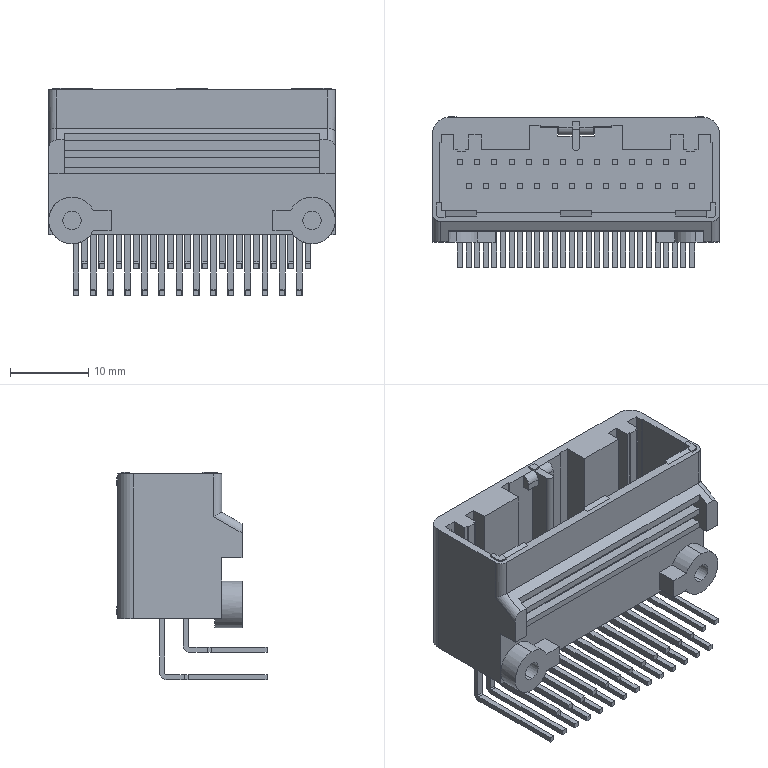Part | SolidWorks | features BaseBody 1 | 1 solid | 653 faces | box 36.7 x 19.2 x 26.52 mm | volume 4801 mm3 | plane 576 | cylinder 77 | commonest cylinder face diameters 0.36 x28 1.64 x28 6 x6 2 x4 2.35 x4 1 x3